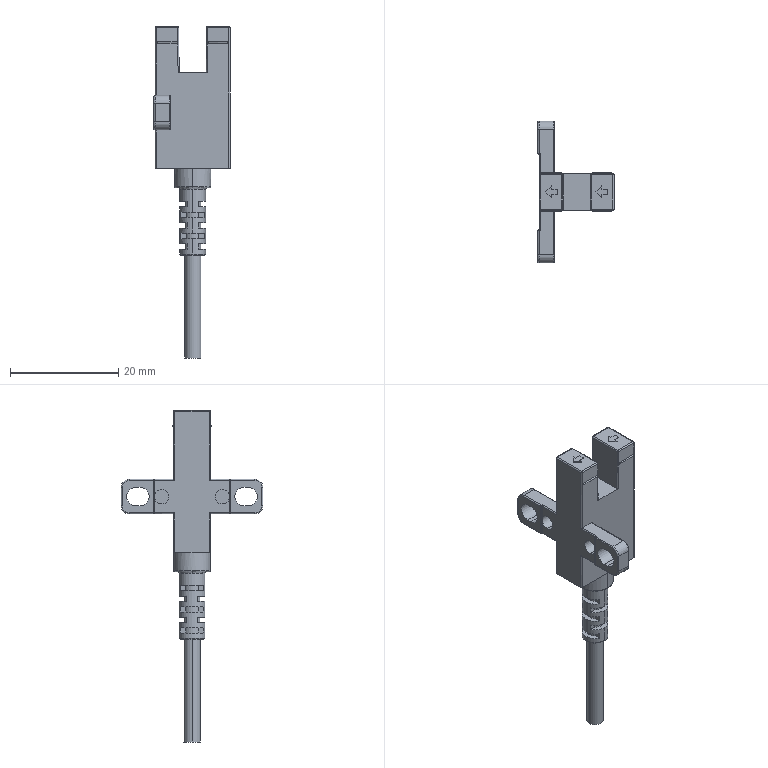Part | STEP file | slot-type photoelectric sensor LU672-5N | 1 solid | 249 faces | box 14.05 x 26.2 x 61.3 mm | volume 1669 mm3 | plane 136 | cylinder 81 | spline 32 | commonest cylinder face diameters 0.4 x40 3 x21 0.3 x4 2.7 x4 3.4 x4 2.8 x2